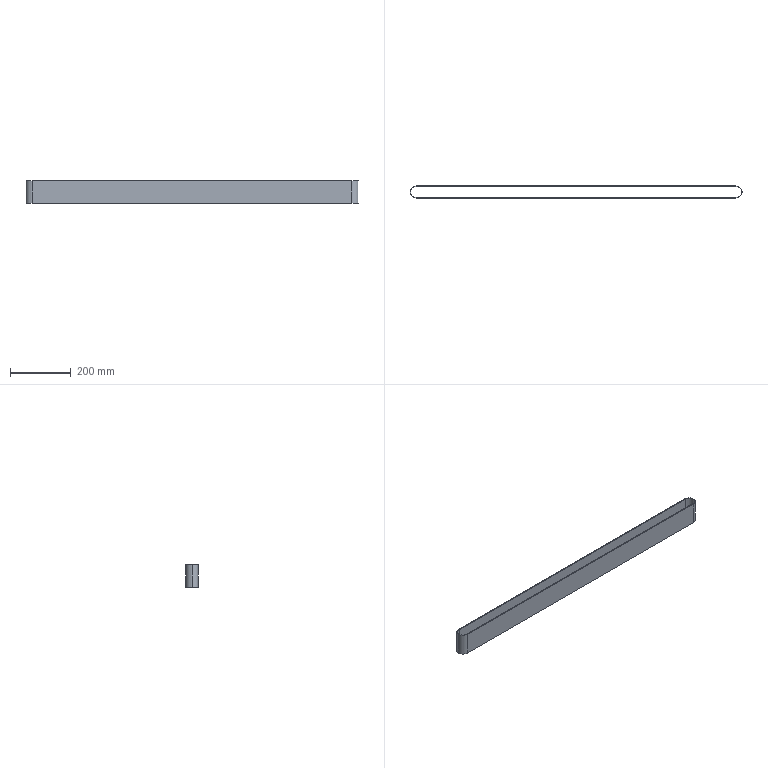Part | STEP file | 1 solid | 12 faces | box 1089 x 40 x 75 mm | volume 332607 mm3 | cylinder 6 | plane 6 | commonest cylinder face diameters 36 x3 40 x3
STEP:
#1=CARTESIAN_POINT('',(0.,0.,0.));
#2=DIRECTION('',(0.,0.,1.));
#3=DIRECTION('',(1.,0.,0.));
#4=AXIS2_PLACEMENT_3D('',#1,#2,#3);
#5=CARTESIAN_POINT('',(-1049.,18.,37.5));
#6=VERTEX_POINT('',#5);
#7=CARTESIAN_POINT('',(-1049.,18.,-37.5));
#8=VERTEX_POINT('',#7);
#9=CARTESIAN_POINT('',(-1049.,18.,37.5));
#10=DIRECTION('',(0.,0.,-1.));
#11=VECTOR('',#10,1.);
#12=LINE('',#9,#11);
#13=CARTESIAN_POINT('',(-1049.,0.,37.5));
#14=DIRECTION('',(0.,0.,-1.));
#15=DIRECTION('',(-1.,0.,0.));
#16=AXIS2_PLACEMENT_3D('',#13,#14,#15);
#17=CYLINDRICAL_SURFACE('',#16,18.);
#18=CARTESIAN_POINT('',(1.571,0.));
#19=DIRECTION('',(0.,1.));
#20=VECTOR('',#19,1.);
#21=LINE('',#18,#20);
#22=(GEOMETRIC_REPRESENTATION_CONTEXT(2)PARAMETRIC_REPRESENTATION_CONTEXT()REPRESENTATION_CONTEXT('',''));
#23=DEFINITIONAL_REPRESENTATION('',(#21),#22);
#24=PCURVE('',#17,#23);
#25=CARTESIAN_POINT('',(-1049.,18.,37.5));
#26=DIRECTION('',(0.,-1.,0.));
#27=DIRECTION('',(1.,0.,0.));
#28=AXIS2_PLACEMENT_3D('',#25,#26,#27);
#29=PLANE('',#28);
#30=CARTESIAN_POINT('',(0.,0.));
#31=DIRECTION('',(0.,-1.));
#32=VECTOR('',#31,1.);
#33=LINE('',#30,#32);
#34=(GEOMETRIC_REPRESENTATION_CONTEXT(2)PARAMETRIC_REPRESENTATION_CONTEXT()REPRESENTATION_CONTEXT('',''));
#35=DEFINITIONAL_REPRESENTATION('',(#33),#34);
#36=PCURVE('',#29,#35);
#37=SURFACE_CURVE('',#12,(#24,#36),.PCURVE_S1.);
#38=EDGE_CURVE('',#6,#8,#37,.T.);
#39=ORIENTED_EDGE('',*,*,#38,.T.);
#40=CARTESIAN_POINT('',(-1067.,0.,-37.5));
#41=VERTEX_POINT('',#40);
#42=CARTESIAN_POINT('',(-1049.,0.,-37.5));
#43=DIRECTION('',(0.,0.,1.));
#44=DIRECTION('',(1.,0.,0.));
#45=AXIS2_PLACEMENT_3D('',#42,#43,#44);
#46=CIRCLE('',#45,18.);
#47=CARTESIAN_POINT('',(3.142,75.));
#48=DIRECTION('',(-1.,0.));
#49=VECTOR('',#48,1.);
#50=LINE('',#47,#49);
#51=(GEOMETRIC_REPRESENTATION_CONTEXT(2)PARAMETRIC_REPRESENTATION_CONTEXT()REPRESENTATION_CONTEXT('',''));
#52=DEFINITIONAL_REPRESENTATION('',(#50),#51);
#53=PCURVE('',#17,#52);
#54=CARTESIAN_POINT('',(0.,0.,-37.5));
#55=DIRECTION('',(0.,0.,-1.));
#56=DIRECTION('',(-1.,0.,0.));
#57=AXIS2_PLACEMENT_3D('',#54,#55,#56);
#58=PLANE('',#57);
#59=CARTESIAN_POINT('',(1031.,0.));
#60=CARTESIAN_POINT('',(1031.,31.177));
#61=CARTESIAN_POINT('',(1058.,15.588));
#62=CARTESIAN_POINT('',(1085.,0.));
#63=CARTESIAN_POINT('',(1058.,-15.588));
#64=CARTESIAN_POINT('',(1031.,-31.177));
#65=CARTESIAN_POINT('',(1031.,0.));
#66=(BOUNDED_CURVE()B_SPLINE_CURVE(2,(#59,#60,#61,#62,#63,#64,#65),.UNSPECIFIED.,.T.,.F.)B_SPLINE_CURVE_WITH_KNOTS((1,2,2,2,2,1),(-2.094,0.,2.094,4.189,6.283,8.378),.UNSPECIFIED.)CURVE()GEOMETRIC_REPRESENTATION_ITEM()RATIONAL_B_SPLINE_CURVE((1.,0.5,1.,0.5,1.,0.5,1.))REPRESENTATION_ITEM(''));
#67=(GEOMETRIC_REPRESENTATION_CONTEXT(2)PARAMETRIC_REPRESENTATION_CONTEXT()REPRESENTATION_CONTEXT('',''));
#68=DEFINITIONAL_REPRESENTATION('',(#66),#67);
#69=PCURVE('',#58,#68);
#70=SURFACE_CURVE('',#46,(#53,#69),.PCURVE_S1.);
#71=EDGE_CURVE('',#8,#41,#70,.T.);
#72=ORIENTED_EDGE('',*,*,#71,.T.);
#73=CARTESIAN_POINT('',(-1067.,0.,37.5));
#74=VERTEX_POINT('',#73);
#75=CARTESIAN_POINT('',(-1067.,0.,37.5));
#76=DIRECTION('',(0.,0.,-1.));
#77=VECTOR('',#76,1.);
#78=LINE('',#75,#77);
#79=CARTESIAN_POINT('',(0.,0.));
#80=DIRECTION('',(0.,1.));
#81=VECTOR('',#80,1.);
#82=LINE('',#79,#81);
#83=(GEOMETRIC_REPRESENTATION_CONTEXT(2)PARAMETRIC_REPRESENTATION_CONTEXT()REPRESENTATION_CONTEXT('',''));
#84=DEFINITIONAL_REPRESENTATION('',(#82),#83);
#85=PCURVE('',#17,#84);
#86=CARTESIAN_POINT('',(-1049.,0.,37.5));
#87=DIRECTION('',(0.,0.,-1.));
#88=DIRECTION('',(-1.,0.,0.));
#89=AXIS2_PLACEMENT_3D('',#86,#87,#88);
#90=CYLINDRICAL_SURFACE('',#89,18.);
#91=CARTESIAN_POINT('',(6.283,0.));
#92=DIRECTION('',(0.,1.));
#93=VECTOR('',#92,1.);
#94=LINE('',#91,#93);
#95=(GEOMETRIC_REPRESENTATION_CONTEXT(2)PARAMETRIC_REPRESENTATION_CONTEXT()REPRESENTATION_CONTEXT('',''));
#96=DEFINITIONAL_REPRESENTATION('',(#94),#95);
#97=PCURVE('',#90,#96);
#98=SURFACE_CURVE('',#78,(#85,#97),.PCURVE_S1.);
#99=EDGE_CURVE('',#74,#41,#98,.T.);
#100=ORIENTED_EDGE('',*,*,#99,.F.);
#101=CARTESIAN_POINT('',(-1049.,0.,37.5));
#102=DIRECTION('',(0.,0.,1.));
#103=DIRECTION('',(1.,0.,0.));
#104=AXIS2_PLACEMENT_3D('',#101,#102,#103);
#105=CIRCLE('',#104,18.);
#106=CARTESIAN_POINT('',(3.142,0.));
#107=DIRECTION('',(-1.,0.));
#108=VECTOR('',#107,1.);
#109=LINE('',#106,#108);
#110=(GEOMETRIC_REPRESENTATION_CONTEXT(2)PARAMETRIC_REPRESENTATION_CONTEXT()REPRESENTATION_CONTEXT('',''));
#111=DEFINITIONAL_REPRESENTATION('',(#109),#110);
#112=PCURVE('',#17,#111);
#113=CARTESIAN_POINT('',(0.,0.,37.5));
#114=DIRECTION('',(0.,0.,-1.));
#115=DIRECTION('',(-1.,0.,0.));
#116=AXIS2_PLACEMENT_3D('',#113,#114,#115);
#117=PLANE('',#116);
#118=CARTESIAN_POINT('',(1031.,0.));
#119=CARTESIAN_POINT('',(1031.,31.177));
#120=CARTESIAN_POINT('',(1058.,15.588));
#121=CARTESIAN_POINT('',(1085.,0.));
#122=CARTESIAN_POINT('',(1058.,-15.588));
#123=CARTESIAN_POINT('',(1031.,-31.177));
#124=CARTESIAN_POINT('',(1031.,0.));
#125=(BOUNDED_CURVE()B_SPLINE_CURVE(2,(#118,#119,#120,#121,#122,#123,#124),.UNSPECIFIED.,.T.,.F.)B_SPLINE_CURVE_WITH_KNOTS((1,2,2,2,2,1),(-2.094,0.,2.094,4.189,6.283,8.378),.UNSPECIFIED.)CURVE()GEOMETRIC_REPRESENTATION_ITEM()RATIONAL_B_SPLINE_CURVE((1.,0.5,1.,0.5,1.,0.5,1.))REPRESENTATION_ITEM(''));
#126=(GEOMETRIC_REPRESENTATION_CONTEXT(2)PARAMETRIC_REPRESENTATION_CONTEXT()REPRESENTATION_CONTEXT('',''));
#127=DEFINITIONAL_REPRESENTATION('',(#125),#126);
#128=PCURVE('',#117,#127);
#129=SURFACE_CURVE('',#105,(#112,#128),.PCURVE_S1.);
#130=EDGE_CURVE('',#6,#74,#129,.T.);
#131=ORIENTED_EDGE('',*,*,#130,.F.);
#132=EDGE_LOOP('',(#39,#72,#100,#131));
#133=FACE_BOUND('',#132,.F.);
#134=ADVANCED_FACE('',(#133),#17,.F.);
#135=CARTESIAN_POINT('',(-1069.,0.,37.5));
#136=VERTEX_POINT('',#135);
#137=CARTESIAN_POINT('',(-1049.,-20.,37.5));
#138=VERTEX_POINT('',#137);
#139=CARTESIAN_POINT('',(-1049.,0.,37.5));
#140=DIRECTION('',(0.,0.,1.));
#141=DIRECTION('',(-1.,0.,0.));
#142=AXIS2_PLACEMENT_3D('',#139,#140,#141);
#143=CIRCLE('',#142,20.);
#144=CARTESIAN_POINT('',(-1049.,0.,37.5));
#145=DIRECTION('',(0.,0.,-1.));
#146=DIRECTION('',(-1.,0.,0.));
#147=AXIS2_PLACEMENT_3D('',#144,#145,#146);
#148=CYLINDRICAL_SURFACE('',#147,20.);
#149=CARTESIAN_POINT('',(6.283,0.));
#150=DIRECTION('',(-1.,0.));
#151=VECTOR('',#150,1.);
#152=LINE('',#149,#151);
#153=(GEOMETRIC_REPRESENTATION_CONTEXT(2)PARAMETRIC_REPRESENTATION_CONTEXT()REPRESENTATION_CONTEXT('',''));
#154=DEFINITIONAL_REPRESENTATION('',(#152),#153);
#155=PCURVE('',#148,#154);
#156=CARTESIAN_POINT('',(1069.,0.));
#157=CARTESIAN_POINT('',(1069.,-34.641));
#158=CARTESIAN_POINT('',(1039.,-17.321));
#159=CARTESIAN_POINT('',(1009.,0.));
#160=CARTESIAN_POINT('',(1039.,17.321));
#161=CARTESIAN_POINT('',(1069.,34.641));
#162=CARTESIAN_POINT('',(1069.,0.));
#163=(BOUNDED_CURVE()B_SPLINE_CURVE(2,(#156,#157,#158,#159,#160,#161,#162),.UNSPECIFIED.,.T.,.F.)B_SPLINE_CURVE_WITH_KNOTS((1,2,2,2,2,1),(-2.094,0.,2.094,4.189,6.283,8.378),.UNSPECIFIED.)CURVE()GEOMETRIC_REPRESENTATION_ITEM()RATIONAL_B_SPLINE_CURVE((1.,0.5,1.,0.5,1.,0.5,1.))REPRESENTATION_ITEM(''));
#164=(GEOMETRIC_REPRESENTATION_CONTEXT(2)PARAMETRIC_REPRESENTATION_CONTEXT()REPRESENTATION_CONTEXT('',''));
#165=DEFINITIONAL_REPRESENTATION('',(#163),#164);
#166=PCURVE('',#117,#165);
#167=SURFACE_CURVE('',#143,(#155,#166),.PCURVE_S1.);
#168=EDGE_CURVE('',#136,#138,#167,.T.);
#169=ORIENTED_EDGE('',*,*,#168,.F.);
#170=CARTESIAN_POINT('',(-1069.,0.,-37.5));
#171=VERTEX_POINT('',#170);
#172=CARTESIAN_POINT('',(-1069.,0.,37.5));
#173=DIRECTION('',(0.,0.,-1.));
#174=VECTOR('',#173,1.);
#175=LINE('',#172,#174);
#176=CARTESIAN_POINT('',(6.283,0.));
#177=DIRECTION('',(0.,1.));
#178=VECTOR('',#177,1.);
#179=LINE('',#176,#178);
#180=(GEOMETRIC_REPRESENTATION_CONTEXT(2)PARAMETRIC_REPRESENTATION_CONTEXT()REPRESENTATION_CONTEXT('',''));
#181=DEFINITIONAL_REPRESENTATION('',(#179),#180);
#182=PCURVE('',#148,#181);
#183=CARTESIAN_POINT('',(-1049.,0.,37.5));
#184=DIRECTION('',(0.,0.,-1.));
#185=DIRECTION('',(-1.,0.,0.));
#186=AXIS2_PLACEMENT_3D('',#183,#184,#185);
#187=CYLINDRICAL_SURFACE('',#186,20.);
#188=CARTESIAN_POINT('',(0.,0.));
#189=DIRECTION('',(0.,1.));
#190=VECTOR('',#189,1.);
#191=LINE('',#188,#190);
#192=(GEOMETRIC_REPRESENTATION_CONTEXT(2)PARAMETRIC_REPRESENTATION_CONTEXT()REPRESENTATION_CONTEXT('',''));
#193=DEFINITIONAL_REPRESENTATION('',(#191),#192);
#194=PCURVE('',#187,#193);
#195=SURFACE_CURVE('',#175,(#182,#194),.PCURVE_S1.);
#196=EDGE_CURVE('',#136,#171,#195,.T.);
#197=ORIENTED_EDGE('',*,*,#196,.T.);
#198=CARTESIAN_POINT('',(-1049.,-20.,-37.5));
#199=VERTEX_POINT('',#198);
#200=CARTESIAN_POINT('',(-1049.,0.,-37.5));
#201=DIRECTION('',(0.,0.,1.));
#202=DIRECTION('',(-1.,0.,0.));
#203=AXIS2_PLACEMENT_3D('',#200,#201,#202);
#204=CIRCLE('',#203,20.);
#205=CARTESIAN_POINT('',(6.283,75.));
#206=DIRECTION('',(-1.,0.));
#207=VECTOR('',#206,1.);
#208=LINE('',#205,#207);
#209=(GEOMETRIC_REPRESENTATION_CONTEXT(2)PARAMETRIC_REPRESENTATION_CONTEXT()REPRESENTATION_CONTEXT('',''));
#210=DEFINITIONAL_REPRESENTATION('',(#208),#209);
#211=PCURVE('',#148,#210);
#212=CARTESIAN_POINT('',(1069.,0.));
#213=CARTESIAN_POINT('',(1069.,-34.641));
#214=CARTESIAN_POINT('',(1039.,-17.321));
#215=CARTESIAN_POINT('',(1009.,0.));
#216=CARTESIAN_POINT('',(1039.,17.321));
#217=CARTESIAN_POINT('',(1069.,34.641));
#218=CARTESIAN_POINT('',(1069.,0.));
#219=(BOUNDED_CURVE()B_SPLINE_CURVE(2,(#212,#213,#214,#215,#216,#217,#218),.UNSPECIFIED.,.T.,.F.)B_SPLINE_CURVE_WITH_KNOTS((1,2,2,2,2,1),(-2.094,0.,2.094,4.189,6.283,8.378),.UNSPECIFIED.)CURVE()GEOMETRIC_REPRESENTATION_ITEM()RATIONAL_B_SPLINE_CURVE((1.,0.5,1.,0.5,1.,0.5,1.))REPRESENTATION_ITEM(''));
#220=(GEOMETRIC_REPRESENTATION_CONTEXT(2)PARAMETRIC_REPRESENTATION_CONTEXT()REPRESENTATION_CONTEXT('',''));
#221=DEFINITIONAL_REPRESENTATION('',(#219),#220);
#222=PCURVE('',#58,#221);
#223=SURFACE_CURVE('',#204,(#211,#222),.PCURVE_S1.);
#224=EDGE_CURVE('',#171,#199,#223,.T.);
#225=ORIENTED_EDGE('',*,*,#224,.T.);
#226=CARTESIAN_POINT('',(-1049.,-20.,37.5));
#227=DIRECTION('',(0.,0.,-1.));
#228=VECTOR('',#227,1.);
#229=LINE('',#226,#228);
#230=CARTESIAN_POINT('',(4.712,0.));
#231=DIRECTION('',(0.,1.));
#232=VECTOR('',#231,1.);
#233=LINE('',#230,#232);
#234=(GEOMETRIC_REPRESENTATION_CONTEXT(2)PARAMETRIC_REPRESENTATION_CONTEXT()REPRESENTATION_CONTEXT('',''));
#235=DEFINITIONAL_REPRESENTATION('',(#233),#234);
#236=PCURVE('',#148,#235);
#237=CARTESIAN_POINT('',(0.,-20.,37.5));
#238=DIRECTION('',(0.,1.,0.));
#239=DIRECTION('',(-1.,0.,0.));
#240=AXIS2_PLACEMENT_3D('',#237,#238,#239);
#241=PLANE('',#240);
#242=CARTESIAN_POINT('',(1049.,0.));
#243=DIRECTION('',(0.,-1.));
#244=VECTOR('',#243,1.);
#245=LINE('',#242,#244);
#246=(GEOMETRIC_REPRESENTATION_CONTEXT(2)PARAMETRIC_REPRESENTATION_CONTEXT()REPRESENTATION_CONTEXT('',''));
#247=DEFINITIONAL_REPRESENTATION('',(#245),#246);
#248=PCURVE('',#241,#247);
#249=SURFACE_CURVE('',#229,(#236,#248),.PCURVE_S1.);
#250=EDGE_CURVE('',#138,#199,#249,.T.);
#251=ORIENTED_EDGE('',*,*,#250,.F.);
#252=EDGE_LOOP('',(#169,#197,#225,#251));
#253=FACE_BOUND('',#252,.T.);
#254=ADVANCED_FACE('',(#253),#148,.T.);
#255=CARTESIAN_POINT('',(0.,-20.,37.5));
#256=VERTEX_POINT('',#255);
#257=CARTESIAN_POINT('',(0.,20.,37.5));
#258=VERTEX_POINT('',#257);
#259=CARTESIAN_POINT('',(0.,0.,37.5));
#260=DIRECTION('',(0.,0.,1.));
#261=DIRECTION('',(-1.,0.,0.));
#262=AXIS2_PLACEMENT_3D('',#259,#260,#261);
#263=CIRCLE('',#262,20.);
#264=CARTESIAN_POINT('',(20.,0.));
#265=CARTESIAN_POINT('',(20.,-34.641));
#266=CARTESIAN_POINT('',(-10.,-17.321));
#267=CARTESIAN_POINT('',(-40.,0.));
#268=CARTESIAN_POINT('',(-10.,17.321));
#269=CARTESIAN_POINT('',(20.,34.641));
#270=CARTESIAN_POINT('',(20.,0.));
#271=(BOUNDED_CURVE()B_SPLINE_CURVE(2,(#264,#265,#266,#267,#268,#269,#270),.UNSPECIFIED.,.T.,.F.)B_SPLINE_CURVE_WITH_KNOTS((1,2,2,2,2,1),(-2.094,0.,2.094,4.189,6.283,8.378),.UNSPECIFIED.)CURVE()GEOMETRIC_REPRESENTATION_ITEM()RATIONAL_B_SPLINE_CURVE((1.,0.5,1.,0.5,1.,0.5,1.))REPRESENTATION_ITEM(''));
#272=(GEOMETRIC_REPRESENTATION_CONTEXT(2)PARAMETRIC_REPRESENTATION_CONTEXT()REPRESENTATION_CONTEXT('',''));
#273=DEFINITIONAL_REPRESENTATION('',(#271),#272);
#274=PCURVE('',#117,#273);
#275=CARTESIAN_POINT('',(0.,0.,37.5));
#276=DIRECTION('',(0.,0.,-1.));
#277=DIRECTION('',(-1.,0.,0.));
#278=AXIS2_PLACEMENT_3D('',#275,#276,#277);
#279=CYLINDRICAL_SURFACE('',#278,20.);
#280=CARTESIAN_POINT('',(6.283,0.));
#281=DIRECTION('',(-1.,0.));
#282=VECTOR('',#281,1.);
#283=LINE('',#280,#282);
#284=(GEOMETRIC_REPRESENTATION_CONTEXT(2)PARAMETRIC_REPRESENTATION_CONTEXT()REPRESENTATION_CONTEXT('',''));
#285=DEFINITIONAL_REPRESENTATION('',(#283),#284);
#286=PCURVE('',#279,#285);
#287=SURFACE_CURVE('',#263,(#274,#286),.PCURVE_S1.);
#288=EDGE_CURVE('',#256,#258,#287,.T.);
#289=ORIENTED_EDGE('',*,*,#288,.T.);
#290=CARTESIAN_POINT('',(-1049.,20.,37.5));
#291=VERTEX_POINT('',#290);
#292=CARTESIAN_POINT('',(0.,20.,37.5));
#293=DIRECTION('',(-1.,0.,0.));
#294=VECTOR('',#293,1.);
#295=LINE('',#292,#294);
#296=CARTESIAN_POINT('',(0.,20.));
#297=DIRECTION('',(1.,0.));
#298=VECTOR('',#297,1.);
#299=LINE('',#296,#298);
#300=(GEOMETRIC_REPRESENTATION_CONTEXT(2)PARAMETRIC_REPRESENTATION_CONTEXT()REPRESENTATION_CONTEXT('',''));
#301=DEFINITIONAL_REPRESENTATION('',(#299),#300);
#302=PCURVE('',#117,#301);
#303=CARTESIAN_POINT('',(0.,20.,37.5));
#304=DIRECTION('',(0.,-1.,0.));
#305=DIRECTION('',(1.,0.,0.));
#306=AXIS2_PLACEMENT_3D('',#303,#304,#305);
#307=PLANE('',#306);
#308=CARTESIAN_POINT('',(0.,0.));
#309=DIRECTION('',(-1.,0.));
#310=VECTOR('',#309,1.);
#311=LINE('',#308,#310);
#312=(GEOMETRIC_REPRESENTATION_CONTEXT(2)PARAMETRIC_REPRESENTATION_CONTEXT()REPRESENTATION_CONTEXT('',''));
#313=DEFINITIONAL_REPRESENTATION('',(#311),#312);
#314=PCURVE('',#307,#313);
#315=SURFACE_CURVE('',#295,(#302,#314),.PCURVE_S1.);
#316=EDGE_CURVE('',#258,#291,#315,.T.);
#317=ORIENTED_EDGE('',*,*,#316,.T.);
#318=CARTESIAN_POINT('',(-1049.,0.,37.5));
#319=DIRECTION('',(0.,0.,1.));
#320=DIRECTION('',(-1.,0.,0.));
#321=AXIS2_PLACEMENT_3D('',#318,#319,#320);
#322=CIRCLE('',#321,20.);
#323=CARTESIAN_POINT('',(1069.,0.));
#324=CARTESIAN_POINT('',(1069.,-34.641));
#325=CARTESIAN_POINT('',(1039.,-17.321));
#326=CARTESIAN_POINT('',(1009.,0.));
#327=CARTESIAN_POINT('',(1039.,17.321));
#328=CARTESIAN_POINT('',(1069.,34.641));
#329=CARTESIAN_POINT('',(1069.,0.));
#330=(BOUNDED_CURVE()B_SPLINE_CURVE(2,(#323,#324,#325,#326,#327,#328,#329),.UNSPECIFIED.,.T.,.F.)B_SPLINE_CURVE_WITH_KNOTS((1,2,2,2,2,1),(-2.094,0.,2.094,4.189,6.283,8.378),.UNSPECIFIED.)CURVE()GEOMETRIC_REPRESENTATION_ITEM()RATIONAL_B_SPLINE_CURVE((1.,0.5,1.,0.5,1.,0.5,1.))REPRESENTATION_ITEM(''));
#331=(GEOMETRIC_REPRESENTATION_CONTEXT(2)PARAMETRIC_REPRESENTATION_CONTEXT()REPRESENTATION_CONTEXT('',''));
#332=DEFINITIONAL_REPRESENTATION('',(#330),#331);
#333=PCURVE('',#117,#332);
#334=CARTESIAN_POINT('',(6.283,0.));
#335=DIRECTION('',(-1.,0.));
#336=VECTOR('',#335,1.);
#337=LINE('',#334,#336);
#338=(GEOMETRIC_REPRESENTATION_CONTEXT(2)PARAMETRIC_REPRESENTATION_CONTEXT()REPRESENTATION_CONTEXT('',''));
#339=DEFINITIONAL_REPRESENTATION('',(#337),#338);
#340=PCURVE('',#187,#339);
#341=SURFACE_CURVE('',#322,(#333,#340),.PCURVE_S1.);
#342=EDGE_CURVE('',#291,#136,#341,.T.);
#343=ORIENTED_EDGE('',*,*,#342,.T.);
#344=ORIENTED_EDGE('',*,*,#168,.T.);
#345=CARTESIAN_POINT('',(0.,-20.,37.5));
#346=DIRECTION('',(1.,0.,0.));
#347=VECTOR('',#346,1.);
#348=LINE('',#345,#347);
#349=CARTESIAN_POINT('',(0.,-20.));
#350=DIRECTION('',(-1.,0.));
#351=VECTOR('',#350,1.);
#352=LINE('',#349,#351);
#353=(GEOMETRIC_REPRESENTATION_CONTEXT(2)PARAMETRIC_REPRESENTATION_CONTEXT()REPRESENTATION_CONTEXT('',''));
#354=DEFINITIONAL_REPRESENTATION('',(#352),#353);
#355=PCURVE('',#117,#354);
#356=CARTESIAN_POINT('',(0.,0.));
#357=DIRECTION('',(-1.,0.));
#358=VECTOR('',#357,1.);
#359=LINE('',#356,#358);
#360=(GEOMETRIC_REPRESENTATION_CONTEXT(2)PARAMETRIC_REPRESENTATION_CONTEXT()REPRESENTATION_CONTEXT('',''));
#361=DEFINITIONAL_REPRESENTATION('',(#359),#360);
#362=PCURVE('',#241,#361);
#363=SURFACE_CURVE('',#348,(#355,#362),.PCURVE_S1.);
#364=EDGE_CURVE('',#138,#256,#363,.T.);
#365=ORIENTED_EDGE('',*,*,#364,.T.);
#366=EDGE_LOOP('',(#289,#317,#343,#344,#365));
#367=FACE_BOUND('',#366,.T.);
#368=CARTESIAN_POINT('',(0.,-18.,37.5));
#369=VERTEX_POINT('',#368);
#370=CARTESIAN_POINT('',(0.,18.,37.5));
#371=VERTEX_POINT('',#370);
#372=CARTESIAN_POINT('',(0.,0.,37.5));
#373=DIRECTION('',(0.,0.,1.));
#374=DIRECTION('',(-1.,0.,0.));
#375=AXIS2_PLACEMENT_3D('',#372,#373,#374);
#376=CIRCLE('',#375,18.);
#377=CARTESIAN_POINT('',(18.,0.));
#378=CARTESIAN_POINT('',(18.,-31.177));
#379=CARTESIAN_POINT('',(-9.,-15.588));
#380=CARTESIAN_POINT('',(-36.,0.));
#381=CARTESIAN_POINT('',(-9.,15.588));
#382=CARTESIAN_POINT('',(18.,31.177));
#383=CARTESIAN_POINT('',(18.,0.));
#384=(BOUNDED_CURVE()B_SPLINE_CURVE(2,(#377,#378,#379,#380,#381,#382,#383),.UNSPECIFIED.,.T.,.F.)B_SPLINE_CURVE_WITH_KNOTS((1,2,2,2,2,1),(-2.094,0.,2.094,4.189,6.283,8.378),.UNSPECIFIED.)CURVE()GEOMETRIC_REPRESENTATION_ITEM()RATIONAL_B_SPLINE_CURVE((1.,0.5,1.,0.5,1.,0.5,1.))REPRESENTATION_ITEM(''));
#385=(GEOMETRIC_REPRESENTATION_CONTEXT(2)PARAMETRIC_REPRESENTATION_CONTEXT()REPRESENTATION_CONTEXT('',''));
#386=DEFINITIONAL_REPRESENTATION('',(#384),#385);
#387=PCURVE('',#117,#386);
#388=CARTESIAN_POINT('',(0.,0.,37.5));
#389=DIRECTION('',(0.,0.,-1.));
#390=DIRECTION('',(-1.,0.,0.));
#391=AXIS2_PLACEMENT_3D('',#388,#389,#390);
#392=CYLINDRICAL_SURFACE('',#391,18.);
#393=CARTESIAN_POINT('',(6.283,0.));
#394=DIRECTION('',(-1.,0.));
#395=VECTOR('',#394,1.);
#396=LINE('',#393,#395);
#397=(GEOMETRIC_REPRESENTATION_CONTEXT(2)PARAMETRIC_REPRESENTATION_CONTEXT()REPRESENTATION_CONTEXT('',''));
#398=DEFINITIONAL_REPRESENTATION('',(#396),#397);
#399=PCURVE('',#392,#398);
#400=SURFACE_CURVE('',#376,(#387,#399),.PCURVE_S1.);
#401=EDGE_CURVE('',#369,#371,#400,.T.);
#402=ORIENTED_EDGE('',*,*,#401,.F.);
#403=CARTESIAN_POINT('',(-1049.,-18.,37.5));
#404=VERTEX_POINT('',#403);
#405=CARTESIAN_POINT('',(0.,-18.,37.5));
#406=DIRECTION('',(1.,0.,0.));
#407=VECTOR('',#406,1.);
#408=LINE('',#405,#407);
#409=CARTESIAN_POINT('',(0.,-18.));
#410=DIRECTION('',(-1.,0.));
#411=VECTOR('',#410,1.);
#412=LINE('',#409,#411);
#413=(GEOMETRIC_REPRESENTATION_CONTEXT(2)PARAMETRIC_REPRESENTATION_CONTEXT()REPRESENTATION_CONTEXT('',''));
#414=DEFINITIONAL_REPRESENTATION('',(#412),#413);
#415=PCURVE('',#117,#414);
#416=CARTESIAN_POINT('',(0.,-18.,37.5));
#417=DIRECTION('',(0.,1.,0.));
#418=DIRECTION('',(-1.,0.,0.));
#419=AXIS2_PLACEMENT_3D('',#416,#417,#418);
#420=PLANE('',#419);
#421=CARTESIAN_POINT('',(0.,0.));
#422=DIRECTION('',(-1.,0.));
#423=VECTOR('',#422,1.);
#424=LINE('',#421,#423);
#425=(GEOMETRIC_REPRESENTATION_CONTEXT(2)PARAMETRIC_REPRESENTATION_CONTEXT()REPRESENTATION_CONTEXT('',''));
#426=DEFINITIONAL_REPRESENTATION('',(#424),#425);
#427=PCURVE('',#420,#426);
#428=SURFACE_CURVE('',#408,(#415,#427),.PCURVE_S1.);
#429=EDGE_CURVE('',#404,#369,#428,.T.);
#430=ORIENTED_EDGE('',*,*,#429,.F.);
#431=CARTESIAN_POINT('',(-1049.,0.,37.5));
#432=DIRECTION('',(0.,0.,1.));
#433=DIRECTION('',(1.,0.,0.));
#434=AXIS2_PLACEMENT_3D('',#431,#432,#433);
#435=CIRCLE('',#434,18.);
#436=CARTESIAN_POINT('',(1031.,0.));
#437=CARTESIAN_POINT('',(1031.,31.177));
#438=CARTESIAN_POINT('',(1058.,15.588));
#439=CARTESIAN_POINT('',(1085.,0.));
#440=CARTESIAN_POINT('',(1058.,-15.588));
#441=CARTESIAN_POINT('',(1031.,-31.177));
#442=CARTESIAN_POINT('',(1031.,0.));
#443=(BOUNDED_CURVE()B_SPLINE_CURVE(2,(#436,#437,#438,#439,#440,#441,#442),.UNSPECIFIED.,.T.,.F.)B_SPLINE_CURVE_WITH_KNOTS((1,2,2,2,2,1),(-2.094,0.,2.094,4.189,6.283,8.378),.UNSPECIFIED.)CURVE()GEOMETRIC_REPRESENTATION_ITEM()RATIONAL_B_SPLINE_CURVE((1.,0.5,1.,0.5,1.,0.5,1.))REPRESENTATION_ITEM(''));
#444=(GEOMETRIC_REPRESENTATION_CONTEXT(2)PARAMETRIC_REPRESENTATION_CONTEXT()REPRESENTATION_CONTEXT('',''));
#445=DEFINITIONAL_REPRESENTATION('',(#443),#444);
#446=PCURVE('',#117,#445);
#447=CARTESIAN_POINT('',(9.425,0.));
#448=DIRECTION('',(-1.,0.));
#449=VECTOR('',#448,1.);
#450=LINE('',#447,#449);
#451=(GEOMETRIC_REPRESENTATION_CONTEXT(2)PARAMETRIC_REPRESENTATION_CONTEXT()REPRESENTATION_CONTEXT('',''));
#452=DEFINITIONAL_REPRESENTATION('',(#450),#451);
#453=PCURVE('',#90,#452);
#454=SURFACE_CURVE('',#435,(#446,#453),.PCURVE_S1.);
#455=EDGE_CURVE('',#74,#404,#454,.T.);
#456=ORIENTED_EDGE('',*,*,#455,.F.);
#457=ORIENTED_EDGE('',*,*,#130,.F.);
#458=CARTESIAN_POINT('',(-1049.,18.,37.5));
#459=DIRECTION('',(-1.,0.,0.));
#460=VECTOR('',#459,1.);
#461=LINE('',#458,#460);
#462=CARTESIAN_POINT('',(1049.,18.));
#463=DIRECTION('',(1.,0.));
#464=VECTOR('',#463,1.);
#465=LINE('',#462,#464);
#466=(GEOMETRIC_REPRESENTATION_CONTEXT(2)PARAMETRIC_REPRESENTATION_CONTEXT()REPRESENTATION_CONTEXT('',''));
#467=DEFINITIONAL_REPRESENTATION('',(#465),#466);
#468=PCURVE('',#117,#467);
#469=CARTESIAN_POINT('',(0.,0.));
#470=DIRECTION('',(-1.,0.));
#471=VECTOR('',#470,1.);
#472=LINE('',#469,#471);
#473=(GEOMETRIC_REPRESENTATION_CONTEXT(2)PARAMETRIC_REPRESENTATION_CONTEXT()REPRESENTATION_CONTEXT('',''));
#474=DEFINITIONAL_REPRESENTATION('',(#472),#473);
#475=PCURVE('',#29,#474);
#476=SURFACE_CURVE('',#461,(#468,#475),.PCURVE_S1.);
#477=EDGE_CURVE('',#371,#6,#476,.T.);
#478=ORIENTED_EDGE('',*,*,#477,.F.);
#479=EDGE_LOOP('',(#402,#430,#456,#457,#478));
#480=FACE_BOUND('',#479,.T.);
#481=ADVANCED_FACE('',(#367,#480),#117,.F.);
#482=CARTESIAN_POINT('',(0.,-20.,-37.5));
#483=VERTEX_POINT('',#482);
#484=CARTESIAN_POINT('',(0.,20.,-37.5));
#485=VERTEX_POINT('',#484);
#486=CARTESIAN_POINT('',(0.,0.,-37.5));
#487=DIRECTION('',(0.,0.,1.));
#488=DIRECTION('',(-1.,0.,0.));
#489=AXIS2_PLACEMENT_3D('',#486,#487,#488);
#490=CIRCLE('',#489,20.);
#491=CARTESIAN_POINT('',(20.,0.));
#492=CARTESIAN_POINT('',(20.,-34.641));
#493=CARTESIAN_POINT('',(-10.,-17.321));
#494=CARTESIAN_POINT('',(-40.,0.));
#495=CARTESIAN_POINT('',(-10.,17.321));
#496=CARTESIAN_POINT('',(20.,34.641));
#497=CARTESIAN_POINT('',(20.,0.));
#498=(BOUNDED_CURVE()B_SPLINE_CURVE(2,(#491,#492,#493,#494,#495,#496,#497),.UNSPECIFIED.,.T.,.F.)B_SPLINE_CURVE_WITH_KNOTS((1,2,2,2,2,1),(-2.094,0.,2.094,4.189,6.283,8.378),.UNSPECIFIED.)CURVE()GEOMETRIC_REPRESENTATION_ITEM()RATIONAL_B_SPLINE_CURVE((1.,0.5,1.,0.5,1.,0.5,1.))REPRESENTATION_ITEM(''));
#499=(GEOMETRIC_REPRESENTATION_CONTEXT(2)PARAMETRIC_REPRESENTATION_CONTEXT()REPRESENTATION_CONTEXT('',''));
#500=DEFINITIONAL_REPRESENTATION('',(#498),#499);
#501=PCURVE('',#58,#500);
#502=CARTESIAN_POINT('',(6.283,75.));
#503=DIRECTION('',(-1.,0.));
#504=VECTOR('',#503,1.);
#505=LINE('',#502,#504);
#506=(GEOMETRIC_REPRESENTATION_CONTEXT(2)PARAMETRIC_REPRESENTATION_CONTEXT()REPRESENTATION_CONTEXT('',''));
#507=DEFINITIONAL_REPRESENTATION('',(#505),#506);
#508=PCURVE('',#279,#507);
#509=SURFACE_CURVE('',#490,(#501,#508),.PCURVE_S1.);
#510=EDGE_CURVE('',#483,#485,#509,.T.);
#511=ORIENTED_EDGE('',*,*,#510,.F.);
#512=CARTESIAN_POINT('',(0.,-20.,-37.5));
#513=DIRECTION('',(1.,0.,0.));
#514=VECTOR('',#513,1.);
#515=LINE('',#512,#514);
#516=CARTESIAN_POINT('',(0.,-20.));
#517=DIRECTION('',(-1.,0.));
#518=VECTOR('',#517,1.);
#519=LINE('',#516,#518);
#520=(GEOMETRIC_REPRESENTATION_CONTEXT(2)PARAMETRIC_REPRESENTATION_CONTEXT()REPRESENTATION_CONTEXT('',''));
#521=DEFINITIONAL_REPRESENTATION('',(#519),#520);
#522=PCURVE('',#58,#521);
#523=CARTESIAN_POINT('',(0.,-75.));
#524=DIRECTION('',(-1.,0.));
#525=VECTOR('',#524,1.);
#526=LINE('',#523,#525);
#527=(GEOMETRIC_REPRESENTATION_CONTEXT(2)PARAMETRIC_REPRESENTATION_CONTEXT()REPRESENTATION_CONTEXT('',''));
#528=DEFINITIONAL_REPRESENTATION('',(#526),#527);
#529=PCURVE('',#241,#528);
#530=SURFACE_CURVE('',#515,(#522,#529),.PCURVE_S1.);
#531=EDGE_CURVE('',#199,#483,#530,.T.);
#532=ORIENTED_EDGE('',*,*,#531,.F.);
#533=ORIENTED_EDGE('',*,*,#224,.F.);
#534=CARTESIAN_POINT('',(-1049.,20.,-37.5));
#535=VERTEX_POINT('',#534);
#536=CARTESIAN_POINT('',(-1049.,0.,-37.5));
#537=DIRECTION('',(0.,0.,1.));
#538=DIRECTION('',(-1.,0.,0.));
#539=AXIS2_PLACEMENT_3D('',#536,#537,#538);
#540=CIRCLE('',#539,20.);
#541=CARTESIAN_POINT('',(1069.,0.));
#542=CARTESIAN_POINT('',(1069.,-34.641));
#543=CARTESIAN_POINT('',(1039.,-17.321));
#544=CARTESIAN_POINT('',(1009.,0.));
#545=CARTESIAN_POINT('',(1039.,17.321));
#546=CARTESIAN_POINT('',(1069.,34.641));
#547=CARTESIAN_POINT('',(1069.,0.));
#548=(BOUNDED_CURVE()B_SPLINE_CURVE(2,(#541,#542,#543,#544,#545,#546,#547),.UNSPECIFIED.,.T.,.F.)B_SPLINE_CURVE_WITH_KNOTS((1,2,2,2,2,1),(-2.094,0.,2.094,4.189,6.283,8.378),.UNSPECIFIED.)CURVE()GEOMETRIC_REPRESENTATION_ITEM()RATIONAL_B_SPLINE_CURVE((1.,0.5,1.,0.5,1.,0.5,1.))REPRESENTATION_ITEM(''));
#549=(GEOMETRIC_REPRESENTATION_CONTEXT(2)PARAMETRIC_REPRESENTATION_CONTEXT()REPRESENTATION_CONTEXT('',''));
#550=DEFINITIONAL_REPRESENTATION('',(#548),#549);
#551=PCURVE('',#58,#550);
#552=CARTESIAN_POINT('',(6.283,75.));
#553=DIRECTION('',(-1.,0.));
#554=VECTOR('',#553,1.);
#555=LINE('',#552,#554);
#556=(GEOMETRIC_REPRESENTATION_CONTEXT(2)PARAMETRIC_REPRESENTATION_CONTEXT()REPRESENTATION_CONTEXT('',''));
#557=DEFINITIONAL_REPRESENTATION('',(#555),#556);
#558=PCURVE('',#187,#557);
#559=SURFACE_CURVE('',#540,(#551,#558),.PCURVE_S1.);
#560=EDGE_CURVE('',#535,#171,#559,.T.);
#561=ORIENTED_EDGE('',*,*,#560,.F.);
#562=CARTESIAN_POINT('',(0.,20.,-37.5));
#563=DIRECTION('',(-1.,0.,0.));
#564=VECTOR('',#563,1.);
#565=LINE('',#562,#564);
#566=CARTESIAN_POINT('',(0.,20.));
#567=DIRECTION('',(1.,0.));
#568=VECTOR('',#567,1.);
#569=LINE('',#566,#568);
#570=(GEOMETRIC_REPRESENTATION_CONTEXT(2)PARAMETRIC_REPRESENTATION_CONTEXT()REPRESENTATION_CONTEXT('',''));
#571=DEFINITIONAL_REPRESENTATION('',(#569),#570);
#572=PCURVE('',#58,#571);
#573=CARTESIAN_POINT('',(0.,-75.));
#574=DIRECTION('',(-1.,0.));
#575=VECTOR('',#574,1.);
#576=LINE('',#573,#575);
#577=(GEOMETRIC_REPRESENTATION_CONTEXT(2)PARAMETRIC_REPRESENTATION_CONTEXT()REPRESENTATION_CONTEXT('',''));
#578=DEFINITIONAL_REPRESENTATION('',(#576),#577);
#579=PCURVE('',#307,#578);
#580=SURFACE_CURVE('',#565,(#572,#579),.PCURVE_S1.);
#581=EDGE_CURVE('',#485,#535,#580,.T.);
#582=ORIENTED_EDGE('',*,*,#581,.F.);
#583=EDGE_LOOP('',(#511,#532,#533,#561,#582));
#584=FACE_BOUND('',#583,.T.);
#585=CARTESIAN_POINT('',(-1049.,-18.,-37.5));
#586=VERTEX_POINT('',#585);
#587=CARTESIAN_POINT('',(0.,-18.,-37.5));
#588=VERTEX_POINT('',#587);
#589=CARTESIAN_POINT('',(0.,-18.,-37.5));
#590=DIRECTION('',(1.,0.,0.));
#591=VECTOR('',#590,1.);
#592=LINE('',#589,#591);
#593=CARTESIAN_POINT('',(0.,-18.));
#594=DIRECTION('',(-1.,0.));
#595=VECTOR('',#594,1.);
#596=LINE('',#593,#595);
#597=(GEOMETRIC_REPRESENTATION_CONTEXT(2)PARAMETRIC_REPRESENTATION_CONTEXT()REPRESENTATION_CONTEXT('',''));
#598=DEFINITIONAL_REPRESENTATION('',(#596),#597);
#599=PCURVE('',#58,#598);
#600=CARTESIAN_POINT('',(0.,-75.));
#601=DIRECTION('',(-1.,0.));
#602=VECTOR('',#601,1.);
#603=LINE('',#600,#602);
#604=(GEOMETRIC_REPRESENTATION_CONTEXT(2)PARAMETRIC_REPRESENTATION_CONTEXT()REPRESENTATION_CONTEXT('',''));
#605=DEFINITIONAL_REPRESENTATION('',(#603),#604);
#606=PCURVE('',#420,#605);
#607=SURFACE_CURVE('',#592,(#599,#606),.PCURVE_S1.);
#608=EDGE_CURVE('',#586,#588,#607,.T.);
#609=ORIENTED_EDGE('',*,*,#608,.T.);
#610=CARTESIAN_POINT('',(0.,18.,-37.5));
#611=VERTEX_POINT('',#610);
#612=CARTESIAN_POINT('',(0.,0.,-37.5));
#613=DIRECTION('',(0.,0.,1.));
#614=DIRECTION('',(-1.,0.,0.));
#615=AXIS2_PLACEMENT_3D('',#612,#613,#614);
#616=CIRCLE('',#615,18.);
#617=CARTESIAN_POINT('',(18.,0.));
#618=CARTESIAN_POINT('',(18.,-31.177));
#619=CARTESIAN_POINT('',(-9.,-15.588));
#620=CARTESIAN_POINT('',(-36.,0.));
#621=CARTESIAN_POINT('',(-9.,15.588));
#622=CARTESIAN_POINT('',(18.,31.177));
#623=CARTESIAN_POINT('',(18.,0.));
#624=(BOUNDED_CURVE()B_SPLINE_CURVE(2,(#617,#618,#619,#620,#621,#622,#623),.UNSPECIFIED.,.T.,.F.)B_SPLINE_CURVE_WITH_KNOTS((1,2,2,2,2,1),(-2.094,0.,2.094,4.189,6.283,8.378),.UNSPECIFIED.)CURVE()GEOMETRIC_REPRESENTATION_ITEM()RATIONAL_B_SPLINE_CURVE((1.,0.5,1.,0.5,1.,0.5,1.))REPRESENTATION_ITEM(''));
#625=(GEOMETRIC_REPRESENTATION_CONTEXT(2)PARAMETRIC_REPRESENTATION_CONTEXT()REPRESENTATION_CONTEXT('',''));
#626=DEFINITIONAL_REPRESENTATION('',(#624),#625);
#627=PCURVE('',#58,#626);
#628=CARTESIAN_POINT('',(6.283,75.));
#629=DIRECTION('',(-1.,0.));
#630=VECTOR('',#629,1.);
#631=LINE('',#628,#630);
#632=(GEOMETRIC_REPRESENTATION_CONTEXT(2)PARAMETRIC_REPRESENTATION_CONTEXT()REPRESENTATION_CONTEXT('',''));
#633=DEFINITIONAL_REPRESENTATION('',(#631),#632);
#634=PCURVE('',#392,#633);
#635=SURFACE_CURVE('',#616,(#627,#634),.PCURVE_S1.);
#636=EDGE_CURVE('',#588,#611,#635,.T.);
#637=ORIENTED_EDGE('',*,*,#636,.T.);
#638=CARTESIAN_POINT('',(-1049.,18.,-37.5));
#639=DIRECTION('',(-1.,0.,0.));
#640=VECTOR('',#639,1.);
#641=LINE('',#638,#640);
#642=CARTESIAN_POINT('',(1049.,18.));
#643=DIRECTION('',(1.,0.));
#644=VECTOR('',#643,1.);
#645=LINE('',#642,#644);
#646=(GEOMETRIC_REPRESENTATION_CONTEXT(2)PARAMETRIC_REPRESENTATION_CONTEXT()REPRESENTATION_CONTEXT('',''));
#647=DEFINITIONAL_REPRESENTATION('',(#645),#646);
#648=PCURVE('',#58,#647);
#649=CARTESIAN_POINT('',(0.,-75.));
#650=DIRECTION('',(-1.,0.));
#651=VECTOR('',#650,1.);
#652=LINE('',#649,#651);
#653=(GEOMETRIC_REPRESENTATION_CONTEXT(2)PARAMETRIC_REPRESENTATION_CONTEXT()REPRESENTATION_CONTEXT('',''));
#654=DEFINITIONAL_REPRESENTATION('',(#652),#653);
#655=PCURVE('',#29,#654);
#656=SURFACE_CURVE('',#641,(#648,#655),.PCURVE_S1.);
#657=EDGE_CURVE('',#611,#8,#656,.T.);
#658=ORIENTED_EDGE('',*,*,#657,.T.);
#659=ORIENTED_EDGE('',*,*,#71,.T.);
#660=CARTESIAN_POINT('',(-1049.,0.,-37.5));
#661=DIRECTION('',(0.,0.,1.));
#662=DIRECTION('',(1.,0.,0.));
#663=AXIS2_PLACEMENT_3D('',#660,#661,#662);
#664=CIRCLE('',#663,18.);
#665=CARTESIAN_POINT('',(1031.,0.));
#666=CARTESIAN_POINT('',(1031.,31.177));
#667=CARTESIAN_POINT('',(1058.,15.588));
#668=CARTESIAN_POINT('',(1085.,0.));
#669=CARTESIAN_POINT('',(1058.,-15.588));
#670=CARTESIAN_POINT('',(1031.,-31.177));
#671=CARTESIAN_POINT('',(1031.,0.));
#672=(BOUNDED_CURVE()B_SPLINE_CURVE(2,(#665,#666,#667,#668,#669,#670,#671),.UNSPECIFIED.,.T.,.F.)B_SPLINE_CURVE_WITH_KNOTS((1,2,2,2,2,1),(-2.094,0.,2.094,4.189,6.283,8.378),.UNSPECIFIED.)CURVE()GEOMETRIC_REPRESENTATION_ITEM()RATIONAL_B_SPLINE_CURVE((1.,0.5,1.,0.5,1.,0.5,1.))REPRESENTATION_ITEM(''));
#673=(GEOMETRIC_REPRESENTATION_CONTEXT(2)PARAMETRIC_REPRESENTATION_CONTEXT()REPRESENTATION_CONTEXT('',''));
#674=DEFINITIONAL_REPRESENTATION('',(#672),#673);
#675=PCURVE('',#58,#674);
#676=CARTESIAN_POINT('',(9.425,75.));
#677=DIRECTION('',(-1.,0.));
#678=VECTOR('',#677,1.);
#679=LINE('',#676,#678);
#680=(GEOMETRIC_REPRESENTATION_CONTEXT(2)PARAMETRIC_REPRESENTATION_CONTEXT()REPRESENTATION_CONTEXT('',''));
#681=DEFINITIONAL_REPRESENTATION('',(#679),#680);
#682=PCURVE('',#90,#681);
#683=SURFACE_CURVE('',#664,(#675,#682),.PCURVE_S1.);
#684=EDGE_CURVE('',#41,#586,#683,.T.);
#685=ORIENTED_EDGE('',*,*,#684,.T.);
#686=EDGE_LOOP('',(#609,#637,#658,#659,#685));
#687=FACE_BOUND('',#686,.T.);
#688=ADVANCED_FACE('',(#584,#687),#58,.T.);
#689=ORIENTED_EDGE('',*,*,#510,.T.);
#690=CARTESIAN_POINT('',(0.,20.,37.5));
#691=DIRECTION('',(0.,0.,-1.));
#692=VECTOR('',#691,1.);
#693=LINE('',#690,#692);
#694=CARTESIAN_POINT('',(1.571,0.));
#695=DIRECTION('',(0.,1.));
#696=VECTOR('',#695,1.);
#697=LINE('',#694,#696);
#698=(GEOMETRIC_REPRESENTATION_CONTEXT(2)PARAMETRIC_REPRESENTATION_CONTEXT()REPRESENTATION_CONTEXT('',''));
#699=DEFINITIONAL_REPRESENTATION('',(#697),#698);
#700=PCURVE('',#279,#699);
#701=CARTESIAN_POINT('',(0.,0.));
#702=DIRECTION('',(0.,-1.));
#703=VECTOR('',#702,1.);
#704=LINE('',#701,#703);
#705=(GEOMETRIC_REPRESENTATION_CONTEXT(2)PARAMETRIC_REPRESENTATION_CONTEXT()REPRESENTATION_CONTEXT('',''));
#706=DEFINITIONAL_REPRESENTATION('',(#704),#705);
#707=PCURVE('',#307,#706);
#708=SURFACE_CURVE('',#693,(#700,#707),.PCURVE_S1.);
#709=EDGE_CURVE('',#258,#485,#708,.T.);
#710=ORIENTED_EDGE('',*,*,#709,.F.);
#711=ORIENTED_EDGE('',*,*,#288,.F.);
#712=CARTESIAN_POINT('',(0.,-20.,37.5));
#713=DIRECTION('',(0.,0.,-1.));
#714=VECTOR('',#713,1.);
#715=LINE('',#712,#714);
#716=CARTESIAN_POINT('',(4.712,0.));
#717=DIRECTION('',(0.,1.));
#718=VECTOR('',#717,1.);
#719=LINE('',#716,#718);
#720=(GEOMETRIC_REPRESENTATION_CONTEXT(2)PARAMETRIC_REPRESENTATION_CONTEXT()REPRESENTATION_CONTEXT('',''));
#721=DEFINITIONAL_REPRESENTATION('',(#719),#720);
#722=PCURVE('',#279,#721);
#723=CARTESIAN_POINT('',(0.,0.));
#724=DIRECTION('',(0.,-1.));
#725=VECTOR('',#724,1.);
#726=LINE('',#723,#725);
#727=(GEOMETRIC_REPRESENTATION_CONTEXT(2)PARAMETRIC_REPRESENTATION_CONTEXT()REPRESENTATION_CONTEXT('',''));
#728=DEFINITIONAL_REPRESENTATION('',(#726),#727);
#729=PCURVE('',#241,#728);
#730=SURFACE_CURVE('',#715,(#722,#729),.PCURVE_S1.);
#731=EDGE_CURVE('',#256,#483,#730,.T.);
#732=ORIENTED_EDGE('',*,*,#731,.T.);
#733=EDGE_LOOP('',(#689,#710,#711,#732));
#734=FACE_BOUND('',#733,.T.);
#735=ADVANCED_FACE('',(#734),#279,.T.);
#736=ORIENTED_EDGE('',*,*,#581,.T.);
#737=CARTESIAN_POINT('',(-1049.,20.,37.5));
#738=DIRECTION('',(0.,0.,-1.));
#739=VECTOR('',#738,1.);
#740=LINE('',#737,#739);
#741=CARTESIAN_POINT('',(-1049.,0.));
#742=DIRECTION('',(0.,-1.));
#743=VECTOR('',#742,1.);
#744=LINE('',#741,#743);
#745=(GEOMETRIC_REPRESENTATION_CONTEXT(2)PARAMETRIC_REPRESENTATION_CONTEXT()REPRESENTATION_CONTEXT('',''));
#746=DEFINITIONAL_REPRESENTATION('',(#744),#745);
#747=PCURVE('',#307,#746);
#748=CARTESIAN_POINT('',(1.571,0.));
#749=DIRECTION('',(0.,1.));
#750=VECTOR('',#749,1.);
#751=LINE('',#748,#750);
#752=(GEOMETRIC_REPRESENTATION_CONTEXT(2)PARAMETRIC_REPRESENTATION_CONTEXT()REPRESENTATION_CONTEXT('',''));
#753=DEFINITIONAL_REPRESENTATION('',(#751),#752);
#754=PCURVE('',#187,#753);
#755=SURFACE_CURVE('',#740,(#747,#754),.PCURVE_S1.);
#756=EDGE_CURVE('',#291,#535,#755,.T.);
#757=ORIENTED_EDGE('',*,*,#756,.F.);
#758=ORIENTED_EDGE('',*,*,#316,.F.);
#759=ORIENTED_EDGE('',*,*,#709,.T.);
#760=EDGE_LOOP('',(#736,#757,#758,#759));
#761=FACE_BOUND('',#760,.T.);
#762=ADVANCED_FACE('',(#761),#307,.F.);
#763=ORIENTED_EDGE('',*,*,#196,.F.);
#764=ORIENTED_EDGE('',*,*,#342,.F.);
#765=ORIENTED_EDGE('',*,*,#756,.T.);
#766=ORIENTED_EDGE('',*,*,#560,.T.);
#767=EDGE_LOOP('',(#763,#764,#765,#766));
#768=FACE_BOUND('',#767,.T.);
#769=ADVANCED_FACE('',(#768),#187,.T.);
#770=ORIENTED_EDGE('',*,*,#531,.T.);
#771=ORIENTED_EDGE('',*,*,#731,.F.);
#772=ORIENTED_EDGE('',*,*,#364,.F.);
#773=ORIENTED_EDGE('',*,*,#250,.T.);
#774=EDGE_LOOP('',(#770,#771,#772,#773));
#775=FACE_BOUND('',#774,.T.);
#776=ADVANCED_FACE('',(#775),#241,.F.);
#777=CARTESIAN_POINT('',(0.,18.,37.5));
#778=DIRECTION('',(0.,0.,-1.));
#779=VECTOR('',#778,1.);
#780=LINE('',#777,#779);
#781=CARTESIAN_POINT('',(1.571,0.));
#782=DIRECTION('',(0.,1.));
#783=VECTOR('',#782,1.);
#784=LINE('',#781,#783);
#785=(GEOMETRIC_REPRESENTATION_CONTEXT(2)PARAMETRIC_REPRESENTATION_CONTEXT()REPRESENTATION_CONTEXT('',''));
#786=DEFINITIONAL_REPRESENTATION('',(#784),#785);
#787=PCURVE('',#392,#786);
#788=CARTESIAN_POINT('',(1049.,0.));
#789=DIRECTION('',(0.,-1.));
#790=VECTOR('',#789,1.);
#791=LINE('',#788,#790);
#792=(GEOMETRIC_REPRESENTATION_CONTEXT(2)PARAMETRIC_REPRESENTATION_CONTEXT()REPRESENTATION_CONTEXT('',''));
#793=DEFINITIONAL_REPRESENTATION('',(#791),#792);
#794=PCURVE('',#29,#793);
#795=SURFACE_CURVE('',#780,(#787,#794),.PCURVE_S1.);
#796=EDGE_CURVE('',#371,#611,#795,.T.);
#797=ORIENTED_EDGE('',*,*,#796,.F.);
#798=ORIENTED_EDGE('',*,*,#401,.F.);
#799=CARTESIAN_POINT('',(0.,-18.,37.5));
#800=DIRECTION('',(0.,0.,-1.));
#801=VECTOR('',#800,1.);
#802=LINE('',#799,#801);
#803=CARTESIAN_POINT('',(4.712,0.));
#804=DIRECTION('',(0.,1.));
#805=VECTOR('',#804,1.);
#806=LINE('',#803,#805);
#807=(GEOMETRIC_REPRESENTATION_CONTEXT(2)PARAMETRIC_REPRESENTATION_CONTEXT()REPRESENTATION_CONTEXT('',''));
#808=DEFINITIONAL_REPRESENTATION('',(#806),#807);
#809=PCURVE('',#392,#808);
#810=CARTESIAN_POINT('',(0.,0.));
#811=DIRECTION('',(0.,-1.));
#812=VECTOR('',#811,1.);
#813=LINE('',#810,#812);
#814=(GEOMETRIC_REPRESENTATION_CONTEXT(2)PARAMETRIC_REPRESENTATION_CONTEXT()REPRESENTATION_CONTEXT('',''));
#815=DEFINITIONAL_REPRESENTATION('',(#813),#814);
#816=PCURVE('',#420,#815);
#817=SURFACE_CURVE('',#802,(#809,#816),.PCURVE_S1.);
#818=EDGE_CURVE('',#369,#588,#817,.T.);
#819=ORIENTED_EDGE('',*,*,#818,.T.);
#820=ORIENTED_EDGE('',*,*,#636,.T.);
#821=EDGE_LOOP('',(#797,#798,#819,#820));
#822=FACE_BOUND('',#821,.F.);
#823=ADVANCED_FACE('',(#822),#392,.F.);
#824=ORIENTED_EDGE('',*,*,#657,.F.);
#825=ORIENTED_EDGE('',*,*,#796,.F.);
#826=ORIENTED_EDGE('',*,*,#477,.T.);
#827=ORIENTED_EDGE('',*,*,#38,.T.);
#828=EDGE_LOOP('',(#824,#825,#826,#827));
#829=FACE_BOUND('',#828,.T.);
#830=ADVANCED_FACE('',(#829),#29,.T.);
#831=ORIENTED_EDGE('',*,*,#684,.T.);
#832=CARTESIAN_POINT('',(-1049.,-18.,37.5));
#833=DIRECTION('',(0.,0.,-1.));
#834=VECTOR('',#833,1.);
#835=LINE('',#832,#834);
#836=CARTESIAN_POINT('',(4.712,0.));
#837=DIRECTION('',(0.,1.));
#838=VECTOR('',#837,1.);
#839=LINE('',#836,#838);
#840=(GEOMETRIC_REPRESENTATION_CONTEXT(2)PARAMETRIC_REPRESENTATION_CONTEXT()REPRESENTATION_CONTEXT('',''));
#841=DEFINITIONAL_REPRESENTATION('',(#839),#840);
#842=PCURVE('',#90,#841);
#843=CARTESIAN_POINT('',(1049.,0.));
#844=DIRECTION('',(0.,-1.));
#845=VECTOR('',#844,1.);
#846=LINE('',#843,#845);
#847=(GEOMETRIC_REPRESENTATION_CONTEXT(2)PARAMETRIC_REPRESENTATION_CONTEXT()REPRESENTATION_CONTEXT('',''));
#848=DEFINITIONAL_REPRESENTATION('',(#846),#847);
#849=PCURVE('',#420,#848);
#850=SURFACE_CURVE('',#835,(#842,#849),.PCURVE_S1.);
#851=EDGE_CURVE('',#404,#586,#850,.T.);
#852=ORIENTED_EDGE('',*,*,#851,.F.);
#853=ORIENTED_EDGE('',*,*,#455,.F.);
#854=ORIENTED_EDGE('',*,*,#99,.T.);
#855=EDGE_LOOP('',(#831,#852,#853,#854));
#856=FACE_BOUND('',#855,.F.);
#857=ADVANCED_FACE('',(#856),#90,.F.);
#858=ORIENTED_EDGE('',*,*,#608,.F.);
#859=ORIENTED_EDGE('',*,*,#851,.F.);
#860=ORIENTED_EDGE('',*,*,#429,.T.);
#861=ORIENTED_EDGE('',*,*,#818,.T.);
#862=EDGE_LOOP('',(#858,#859,#860,#861));
#863=FACE_BOUND('',#862,.T.);
#864=ADVANCED_FACE('',(#863),#420,.T.);
#865=CLOSED_SHELL('',(#134,#254,#481,#688,#735,#762,#769,#776,#823,#830,#857,#864));
#866=MANIFOLD_SOLID_BREP('',#865);
#867=(LENGTH_UNIT()NAMED_UNIT(*)SI_UNIT(.MILLI.,.METRE.));
#868=UNCERTAINTY_MEASURE_WITH_UNIT(LENGTH_MEASURE(0.0000001),#867,'','');
#869=(NAMED_UNIT(*)PLANE_ANGLE_UNIT()SI_UNIT($,.RADIAN.));
#870=(NAMED_UNIT(*)SI_UNIT($,.STERADIAN.)SOLID_ANGLE_UNIT());
#871=(GEOMETRIC_REPRESENTATION_CONTEXT(3)GLOBAL_UNCERTAINTY_ASSIGNED_CONTEXT((#868))GLOBAL_UNIT_ASSIGNED_CONTEXT((#867,#869,#870))REPRESENTATION_CONTEXT('',''));
#872=ADVANCED_BREP_SHAPE_REPRESENTATION('',(#4,#866),#871);